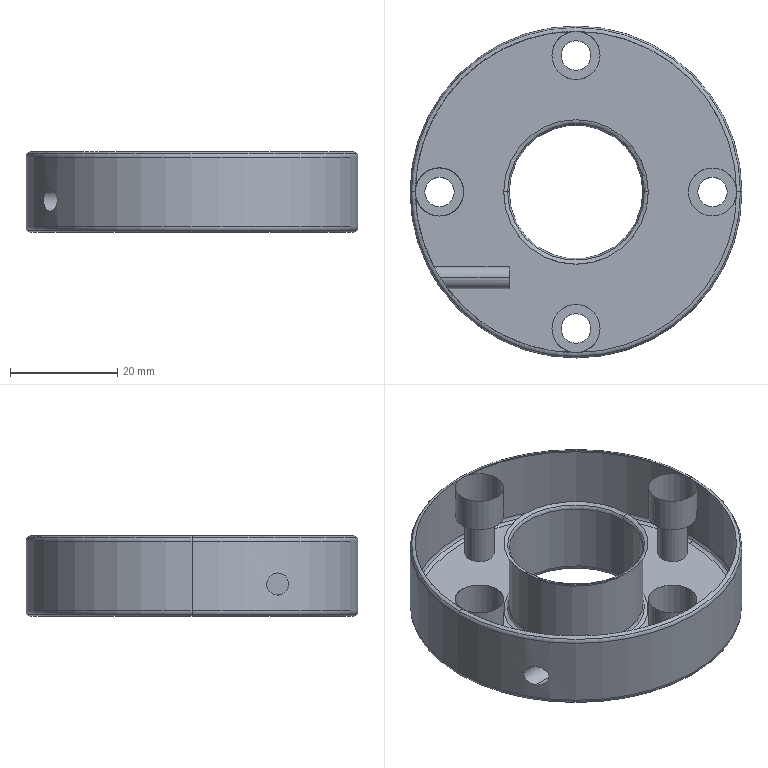Part | NX | features BREP 1 | 1 solid | 45 faces | box 62 x 62 x 15 mm | volume 35156 mm3 | cylinder 22 | torus 16 | plane 7 | commonest cylinder face diameters 5.5 x8 9 x8 4.134 x2 25 x2 62 x2
STEP:
#1=CARTESIAN_POINT('',(4.5,25.5,-6.5));
#2=VERTEX_POINT('',#1);
#3=CARTESIAN_POINT('',(-4.5,25.5,-6.5));
#4=VERTEX_POINT('',#3);
#5=CARTESIAN_POINT('',(0.,25.5,-6.5));
#6=DIRECTION('',(0.,0.,1.));
#7=DIRECTION('',(1.,0.,0.));
#8=AXIS2_PLACEMENT_3D('',#5,#6,#7);
#9=CIRCLE('',#8,4.5);
#10=EDGE_CURVE('',#2,#4,#9,.T.);
#11=ORIENTED_EDGE('',*,*,#10,.T.);
#12=CARTESIAN_POINT('',(0.,25.5,-6.5));
#13=DIRECTION('',(0.,0.,1.));
#14=DIRECTION('',(-1.,0.,0.));
#15=AXIS2_PLACEMENT_3D('',#12,#13,#14);
#16=CIRCLE('',#15,4.5);
#17=EDGE_CURVE('',#4,#2,#16,.T.);
#18=ORIENTED_EDGE('',*,*,#17,.T.);
#19=EDGE_LOOP('',(#11,#18));
#20=FACE_BOUND('',#19,.T.);
#21=CARTESIAN_POINT('',(2.75,25.5,-6.5));
#22=VERTEX_POINT('',#21);
#23=CARTESIAN_POINT('',(-2.75,25.5,-6.5));
#24=VERTEX_POINT('',#23);
#25=CARTESIAN_POINT('',(0.,25.5,-6.5));
#26=DIRECTION('',(0.,0.,-1.));
#27=DIRECTION('',(1.,0.,0.));
#28=AXIS2_PLACEMENT_3D('',#25,#26,#27);
#29=CIRCLE('',#28,2.75);
#30=EDGE_CURVE('',#22,#24,#29,.T.);
#31=ORIENTED_EDGE('',*,*,#30,.T.);
#32=CARTESIAN_POINT('',(0.,25.5,-6.5));
#33=DIRECTION('',(0.,0.,-1.));
#34=DIRECTION('',(-1.,0.,0.));
#35=AXIS2_PLACEMENT_3D('',#32,#33,#34);
#36=CIRCLE('',#35,2.75);
#37=EDGE_CURVE('',#24,#22,#36,.T.);
#38=ORIENTED_EDGE('',*,*,#37,.T.);
#39=EDGE_LOOP('',(#31,#38));
#40=FACE_BOUND('',#39,.T.);
#41=CARTESIAN_POINT('',(0.,30.,-6.5));
#42=DIRECTION('',(0.,0.,1.));
#43=DIRECTION('',(1.,0.,0.));
#44=AXIS2_PLACEMENT_3D('',#41,#42,#43);
#45=PLANE('',#44);
#46=ADVANCED_FACE('',(#20,#40),#45,.T.);
#47=CARTESIAN_POINT('',(4.5,25.5,0.));
#48=VERTEX_POINT('',#47);
#49=CARTESIAN_POINT('',(4.5,25.5,-6.5));
#50=DIRECTION('',(-0.000000009,-0.000000315,1.));
#51=VECTOR('',#50,1000.);
#52=LINE('',#49,#51);
#53=EDGE_CURVE('',#48,#2,#52,.F.);
#54=ORIENTED_EDGE('',*,*,#53,.T.);
#55=ORIENTED_EDGE('',*,*,#17,.F.);
#56=CARTESIAN_POINT('',(-4.5,25.5,0.));
#57=VERTEX_POINT('',#56);
#58=CARTESIAN_POINT('',(-4.5,25.5,-6.5));
#59=DIRECTION('',(0.,0.,1.));
#60=VECTOR('',#59,1000.);
#61=LINE('',#58,#60);
#62=EDGE_CURVE('',#57,#4,#61,.F.);
#63=ORIENTED_EDGE('',*,*,#62,.F.);
#64=CARTESIAN_POINT('',(0.,25.5,0.));
#65=DIRECTION('',(0.,0.,-1.));
#66=DIRECTION('',(1.,-0.000001366,0.));
#67=AXIS2_PLACEMENT_3D('',#64,#65,#66);
#68=CIRCLE('',#67,4.5);
#69=EDGE_CURVE('',#48,#57,#68,.T.);
#70=ORIENTED_EDGE('',*,*,#69,.F.);
#71=EDGE_LOOP('',(#54,#55,#63,#70));
#72=FACE_BOUND('',#71,.T.);
#73=CARTESIAN_POINT('',(0.,25.5,-6.5));
#74=DIRECTION('',(0.,0.,1.));
#75=DIRECTION('',(-1.,0.,0.));
#76=AXIS2_PLACEMENT_3D('',#73,#74,#75);
#77=CYLINDRICAL_SURFACE('',#76,4.5);
#78=ADVANCED_FACE('',(#72),#77,.F.);
#79=CARTESIAN_POINT('',(0.,30.,0.));
#80=VERTEX_POINT('',#79);
#81=CARTESIAN_POINT('',(0.,25.5,0.));
#82=DIRECTION('',(0.,0.,-1.));
#83=DIRECTION('',(-1.,0.,0.));
#84=AXIS2_PLACEMENT_3D('',#81,#82,#83);
#85=CIRCLE('',#84,4.5);
#86=EDGE_CURVE('',#57,#80,#85,.T.);
#87=ORIENTED_EDGE('',*,*,#86,.T.);
#88=CARTESIAN_POINT('',(-30.,0.,0.));
#89=VERTEX_POINT('',#88);
#90=CARTESIAN_POINT('',(0.,0.,0.));
#91=DIRECTION('',(0.,0.,1.));
#92=DIRECTION('',(0.,1.,0.));
#93=AXIS2_PLACEMENT_3D('',#90,#91,#92);
#94=CIRCLE('',#93,30.);
#95=EDGE_CURVE('',#80,#89,#94,.T.);
#96=ORIENTED_EDGE('',*,*,#95,.T.);
#97=CARTESIAN_POINT('',(-21.,0.,0.));
#98=VERTEX_POINT('',#97);
#99=CARTESIAN_POINT('',(-25.5,0.,0.));
#100=DIRECTION('',(0.,0.,-1.));
#101=DIRECTION('',(-1.,0.,0.));
#102=AXIS2_PLACEMENT_3D('',#99,#100,#101);
#103=CIRCLE('',#102,4.5);
#104=EDGE_CURVE('',#89,#98,#103,.T.);
#105=ORIENTED_EDGE('',*,*,#104,.T.);
#106=CARTESIAN_POINT('',(-25.5,0.,0.));
#107=DIRECTION('',(0.,0.,-1.));
#108=DIRECTION('',(1.,0.,0.));
#109=AXIS2_PLACEMENT_3D('',#106,#107,#108);
#110=CIRCLE('',#109,4.5);
#111=EDGE_CURVE('',#98,#89,#110,.T.);
#112=ORIENTED_EDGE('',*,*,#111,.T.);
#113=CARTESIAN_POINT('',(0.,-30.,0.));
#114=VERTEX_POINT('',#113);
#115=CARTESIAN_POINT('',(0.,0.,0.));
#116=DIRECTION('',(0.,0.,1.));
#117=DIRECTION('',(-1.,0.,0.));
#118=AXIS2_PLACEMENT_3D('',#115,#116,#117);
#119=CIRCLE('',#118,30.);
#120=EDGE_CURVE('',#89,#114,#119,.T.);
#121=ORIENTED_EDGE('',*,*,#120,.T.);
#122=CARTESIAN_POINT('',(-4.5,-25.5,0.));
#123=VERTEX_POINT('',#122);
#124=CARTESIAN_POINT('',(0.,-25.5,0.));
#125=DIRECTION('',(0.,0.,-1.));
#126=DIRECTION('',(0.,-1.,0.));
#127=AXIS2_PLACEMENT_3D('',#124,#125,#126);
#128=CIRCLE('',#127,4.5);
#129=EDGE_CURVE('',#114,#123,#128,.T.);
#130=ORIENTED_EDGE('',*,*,#129,.T.);
#131=CARTESIAN_POINT('',(4.5,-25.5,0.));
#132=VERTEX_POINT('',#131);
#133=CARTESIAN_POINT('',(0.,-25.5,0.));
#134=DIRECTION('',(0.,0.,-1.));
#135=DIRECTION('',(-1.,0.,0.));
#136=AXIS2_PLACEMENT_3D('',#133,#134,#135);
#137=CIRCLE('',#136,4.5);
#138=EDGE_CURVE('',#123,#132,#137,.T.);
#139=ORIENTED_EDGE('',*,*,#138,.T.);
#140=CARTESIAN_POINT('',(0.,-25.5,0.));
#141=DIRECTION('',(0.,0.,-1.));
#142=DIRECTION('',(1.,0.,0.));
#143=AXIS2_PLACEMENT_3D('',#140,#141,#142);
#144=CIRCLE('',#143,4.5);
#145=EDGE_CURVE('',#132,#114,#144,.T.);
#146=ORIENTED_EDGE('',*,*,#145,.T.);
#147=CARTESIAN_POINT('',(30.,0.,0.));
#148=VERTEX_POINT('',#147);
#149=CARTESIAN_POINT('',(0.,0.,0.));
#150=DIRECTION('',(0.,0.,1.));
#151=DIRECTION('',(0.,-1.,0.));
#152=AXIS2_PLACEMENT_3D('',#149,#150,#151);
#153=CIRCLE('',#152,30.);
#154=EDGE_CURVE('',#114,#148,#153,.T.);
#155=ORIENTED_EDGE('',*,*,#154,.T.);
#156=CARTESIAN_POINT('',(21.,0.,0.));
#157=VERTEX_POINT('',#156);
#158=CARTESIAN_POINT('',(25.5,0.,0.));
#159=DIRECTION('',(0.,0.,-1.));
#160=DIRECTION('',(1.,0.,0.));
#161=AXIS2_PLACEMENT_3D('',#158,#159,#160);
#162=CIRCLE('',#161,4.5);
#163=EDGE_CURVE('',#148,#157,#162,.T.);
#164=ORIENTED_EDGE('',*,*,#163,.T.);
#165=CARTESIAN_POINT('',(25.5,0.,0.));
#166=DIRECTION('',(0.,0.,-1.));
#167=DIRECTION('',(-1.,0.,0.));
#168=AXIS2_PLACEMENT_3D('',#165,#166,#167);
#169=CIRCLE('',#168,4.5);
#170=EDGE_CURVE('',#157,#148,#169,.T.);
#171=ORIENTED_EDGE('',*,*,#170,.T.);
#172=CARTESIAN_POINT('',(0.,0.,0.));
#173=DIRECTION('',(0.,0.,1.));
#174=DIRECTION('',(1.,0.,0.));
#175=AXIS2_PLACEMENT_3D('',#172,#173,#174);
#176=CIRCLE('',#175,30.);
#177=EDGE_CURVE('',#148,#80,#176,.T.);
#178=ORIENTED_EDGE('',*,*,#177,.T.);
#179=CARTESIAN_POINT('',(0.,25.5,0.));
#180=DIRECTION('',(0.,0.,-1.));
#181=DIRECTION('',(0.,1.,0.));
#182=AXIS2_PLACEMENT_3D('',#179,#180,#181);
#183=CIRCLE('',#182,4.5);
#184=EDGE_CURVE('',#80,#48,#183,.T.);
#185=ORIENTED_EDGE('',*,*,#184,.T.);
#186=ORIENTED_EDGE('',*,*,#69,.T.);
#187=EDGE_LOOP('',(#87,#96,#105,#112,#121,#130,#139,#146,#155,#164,#171,#178,#185,#186));
#188=FACE_BOUND('',#187,.T.);
#189=CARTESIAN_POINT('',(13.5,0.,0.));
#190=VERTEX_POINT('',#189);
#191=CARTESIAN_POINT('',(-13.5,0.,0.));
#192=VERTEX_POINT('',#191);
#193=CARTESIAN_POINT('',(0.,0.,0.));
#194=DIRECTION('',(0.,0.,-1.));
#195=DIRECTION('',(1.,0.,0.));
#196=AXIS2_PLACEMENT_3D('',#193,#194,#195);
#197=CIRCLE('',#196,13.5);
#198=EDGE_CURVE('',#190,#192,#197,.T.);
#199=ORIENTED_EDGE('',*,*,#198,.T.);
#200=CARTESIAN_POINT('',(0.,0.,0.));
#201=DIRECTION('',(0.,0.,-1.));
#202=DIRECTION('',(-1.,0.,0.));
#203=AXIS2_PLACEMENT_3D('',#200,#201,#202);
#204=CIRCLE('',#203,13.5);
#205=EDGE_CURVE('',#192,#190,#204,.T.);
#206=ORIENTED_EDGE('',*,*,#205,.T.);
#207=EDGE_LOOP('',(#199,#206));
#208=FACE_BOUND('',#207,.T.);
#209=CARTESIAN_POINT('',(0.,30.,0.));
#210=DIRECTION('',(0.,0.,1.));
#211=DIRECTION('',(1.,0.,0.));
#212=AXIS2_PLACEMENT_3D('',#209,#210,#211);
#213=PLANE('',#212);
#214=ADVANCED_FACE('',(#188,#208),#213,.T.);
#215=ORIENTED_EDGE('',*,*,#62,.T.);
#216=ORIENTED_EDGE('',*,*,#10,.F.);
#217=ORIENTED_EDGE('',*,*,#53,.F.);
#218=ORIENTED_EDGE('',*,*,#184,.F.);
#219=ORIENTED_EDGE('',*,*,#86,.F.);
#220=EDGE_LOOP('',(#215,#216,#217,#218,#219));
#221=FACE_BOUND('',#220,.T.);
#222=CARTESIAN_POINT('',(0.,25.5,-6.5));
#223=DIRECTION('',(0.,0.,1.));
#224=DIRECTION('',(-1.,0.,0.));
#225=AXIS2_PLACEMENT_3D('',#222,#223,#224);
#226=CYLINDRICAL_SURFACE('',#225,4.5);
#227=ADVANCED_FACE('',(#221),#226,.F.);
#228=ORIENTED_EDGE('',*,*,#177,.F.);
#229=CARTESIAN_POINT('',(30.707,0.,-0.2929));
#230=VERTEX_POINT('',#229);
#231=CARTESIAN_POINT('',(30.,0.,-1.));
#232=DIRECTION('',(0.,1.,0.));
#233=DIRECTION('',(0.,0.,1.));
#234=AXIS2_PLACEMENT_3D('',#231,#232,#233);
#235=CIRCLE('',#234,1.);
#236=EDGE_CURVE('',#230,#148,#235,.F.);
#237=ORIENTED_EDGE('',*,*,#236,.F.);
#238=CARTESIAN_POINT('',(-30.707,0.,-0.2929));
#239=VERTEX_POINT('',#238);
#240=CARTESIAN_POINT('',(0.,0.,-0.2929));
#241=DIRECTION('',(0.,0.,-1.));
#242=DIRECTION('',(-1.,0.,0.));
#243=AXIS2_PLACEMENT_3D('',#240,#241,#242);
#244=CIRCLE('',#243,30.707);
#245=EDGE_CURVE('',#239,#230,#244,.T.);
#246=ORIENTED_EDGE('',*,*,#245,.F.);
#247=CARTESIAN_POINT('',(-30.,0.,-1.));
#248=DIRECTION('',(0.,-1.,0.));
#249=DIRECTION('',(0.,0.,1.));
#250=AXIS2_PLACEMENT_3D('',#247,#248,#249);
#251=CIRCLE('',#250,1.);
#252=EDGE_CURVE('',#239,#89,#251,.F.);
#253=ORIENTED_EDGE('',*,*,#252,.T.);
#254=ORIENTED_EDGE('',*,*,#95,.F.);
#255=EDGE_LOOP('',(#228,#237,#246,#253,#254));
#256=FACE_BOUND('',#255,.T.);
#257=CARTESIAN_POINT('',(0.,0.,-1.));
#258=DIRECTION('',(0.,0.,-1.));
#259=DIRECTION('',(-1.,0.,0.));
#260=AXIS2_PLACEMENT_3D('',#257,#258,#259);
#261=TOROIDAL_SURFACE('',#260,30.,1.);
#262=ADVANCED_FACE('',(#256),#261,.T.);
#263=ORIENTED_EDGE('',*,*,#120,.F.);
#264=ORIENTED_EDGE('',*,*,#252,.F.);
#265=CARTESIAN_POINT('',(0.,0.,-0.2929));
#266=DIRECTION('',(0.,0.,-1.));
#267=DIRECTION('',(1.,0.,0.));
#268=AXIS2_PLACEMENT_3D('',#265,#266,#267);
#269=CIRCLE('',#268,30.707);
#270=EDGE_CURVE('',#230,#239,#269,.T.);
#271=ORIENTED_EDGE('',*,*,#270,.F.);
#272=ORIENTED_EDGE('',*,*,#236,.T.);
#273=ORIENTED_EDGE('',*,*,#154,.F.);
#274=EDGE_LOOP('',(#263,#264,#271,#272,#273));
#275=FACE_BOUND('',#274,.T.);
#276=CARTESIAN_POINT('',(0.,0.,-1.));
#277=DIRECTION('',(0.,0.,-1.));
#278=DIRECTION('',(-1.,0.,0.));
#279=AXIS2_PLACEMENT_3D('',#276,#277,#278);
#280=TOROIDAL_SURFACE('',#279,30.,1.);
#281=ADVANCED_FACE('',(#275),#280,.T.);
#282=CARTESIAN_POINT('',(31.,0.,-1.));
#283=VERTEX_POINT('',#282);
#284=CARTESIAN_POINT('',(30.,0.,-1.));
#285=DIRECTION('',(0.,1.,0.));
#286=DIRECTION('',(0.7071,0.,0.7071));
#287=AXIS2_PLACEMENT_3D('',#284,#285,#286);
#288=CIRCLE('',#287,1.);
#289=EDGE_CURVE('',#283,#230,#288,.F.);
#290=ORIENTED_EDGE('',*,*,#289,.T.);
#291=ORIENTED_EDGE('',*,*,#270,.T.);
#292=CARTESIAN_POINT('',(-31.,0.,-1.));
#293=VERTEX_POINT('',#292);
#294=CARTESIAN_POINT('',(-30.,0.,-1.));
#295=DIRECTION('',(0.,-1.,0.));
#296=DIRECTION('',(-0.7071,0.,0.7071));
#297=AXIS2_PLACEMENT_3D('',#294,#295,#296);
#298=CIRCLE('',#297,1.);
#299=EDGE_CURVE('',#293,#239,#298,.F.);
#300=ORIENTED_EDGE('',*,*,#299,.F.);
#301=CARTESIAN_POINT('',(0.,0.,-1.));
#302=DIRECTION('',(0.,0.,1.));
#303=DIRECTION('',(-1.,0.,0.));
#304=AXIS2_PLACEMENT_3D('',#301,#302,#303);
#305=CIRCLE('',#304,31.);
#306=EDGE_CURVE('',#293,#283,#305,.T.);
#307=ORIENTED_EDGE('',*,*,#306,.T.);
#308=EDGE_LOOP('',(#290,#291,#300,#307));
#309=FACE_BOUND('',#308,.T.);
#310=CARTESIAN_POINT('',(0.,0.,-1.));
#311=DIRECTION('',(0.,0.,-1.));
#312=DIRECTION('',(-1.,0.,0.));
#313=AXIS2_PLACEMENT_3D('',#310,#311,#312);
#314=TOROIDAL_SURFACE('',#313,30.,1.);
#315=ADVANCED_FACE('',(#309),#314,.T.);
#316=CARTESIAN_POINT('',(31.,0.,-14.));
#317=VERTEX_POINT('',#316);
#318=CARTESIAN_POINT('',(31.,0.,-14.));
#319=DIRECTION('',(0.,0.,1.));
#320=VECTOR('',#319,1000.);
#321=LINE('',#318,#320);
#322=EDGE_CURVE('',#283,#317,#321,.F.);
#323=ORIENTED_EDGE('',*,*,#322,.F.);
#324=ORIENTED_EDGE('',*,*,#306,.F.);
#325=CARTESIAN_POINT('',(-31.,0.,-14.));
#326=VERTEX_POINT('',#325);
#327=CARTESIAN_POINT('',(-31.,0.,-14.));
#328=DIRECTION('',(0.,0.,1.));
#329=VECTOR('',#328,1000.);
#330=LINE('',#327,#329);
#331=EDGE_CURVE('',#293,#326,#330,.F.);
#332=ORIENTED_EDGE('',*,*,#331,.T.);
#333=CARTESIAN_POINT('',(0.,0.,-14.));
#334=DIRECTION('',(0.,0.,-1.));
#335=DIRECTION('',(1.,0.,0.));
#336=AXIS2_PLACEMENT_3D('',#333,#334,#335);
#337=CIRCLE('',#336,31.);
#338=EDGE_CURVE('',#317,#326,#337,.T.);
#339=ORIENTED_EDGE('',*,*,#338,.F.);
#340=EDGE_LOOP('',(#323,#324,#332,#339));
#341=FACE_BOUND('',#340,.T.);
#342=CARTESIAN_POINT('',(-26.552,-16.,-11.067));
#343=VERTEX_POINT('',#342);
#344=CARTESIAN_POINT('',(-26.506,-16.075,-11.066));
#345=VERTEX_POINT('',#344);
#346=CARTESIAN_POINT('',(-26.552,-16.,-11.067));
#347=CARTESIAN_POINT('',(-26.547,-16.008,-11.067));
#348=CARTESIAN_POINT('',(-26.537,-16.025,-11.067));
#349=CARTESIAN_POINT('',(-26.521,-16.05,-11.066));
#350=CARTESIAN_POINT('',(-26.511,-16.067,-11.066));
#351=CARTESIAN_POINT('',(-26.506,-16.075,-11.066));
#352=B_SPLINE_CURVE_WITH_KNOTS('',3,(#346,#347,#348,#349,#350,#351),.UNSPECIFIED.,.F.,.F.,(4,1,1,4),(0.,0.3333,0.6667,1.),.UNSPECIFIED.);
#353=EDGE_CURVE('',#343,#345,#352,.T.);
#354=ORIENTED_EDGE('',*,*,#353,.F.);
#355=CARTESIAN_POINT('',(-26.552,-16.,-6.933));
#356=VERTEX_POINT('',#355);
#357=CARTESIAN_POINT('',(-26.552,-16.,-11.067));
#358=CARTESIAN_POINT('',(-26.906,-15.413,-11.067));
#359=CARTESIAN_POINT('',(-27.511,-14.308,-10.535));
#360=CARTESIAN_POINT('',(-27.784,-13.744,-8.997));
#361=CARTESIAN_POINT('',(-27.507,-14.315,-7.458));
#362=CARTESIAN_POINT('',(-26.903,-15.417,-6.933));
#363=CARTESIAN_POINT('',(-26.552,-16.,-6.933));
#364=B_SPLINE_CURVE_WITH_KNOTS('',3,(#357,#358,#359,#360,#361,#362,#363),.UNSPECIFIED.,.F.,.F.,(4,1,1,1,4),(0.,0.25,0.5,0.75,1.),.UNSPECIFIED.);
#365=EDGE_CURVE('',#356,#343,#364,.F.);
#366=ORIENTED_EDGE('',*,*,#365,.F.);
#367=CARTESIAN_POINT('',(-26.552,-16.,-6.933));
#368=CARTESIAN_POINT('',(-26.198,-16.588,-6.933));
#369=CARTESIAN_POINT('',(-25.449,-17.721,-7.498));
#370=CARTESIAN_POINT('',(-25.069,-18.23,-8.97));
#371=CARTESIAN_POINT('',(-25.421,-17.758,-10.451));
#372=CARTESIAN_POINT('',(-26.15,-16.662,-11.044));
#373=CARTESIAN_POINT('',(-26.506,-16.075,-11.066));
#374=B_SPLINE_CURVE_WITH_KNOTS('',3,(#367,#368,#369,#370,#371,#372,#373),.UNSPECIFIED.,.F.,.F.,(4,1,1,1,4),(0.,0.25,0.5,0.75,1.),.UNSPECIFIED.);
#375=EDGE_CURVE('',#345,#356,#374,.F.);
#376=ORIENTED_EDGE('',*,*,#375,.F.);
#377=EDGE_LOOP('',(#354,#366,#376));
#378=FACE_BOUND('',#377,.T.);
#379=CARTESIAN_POINT('',(0.,0.,-50.));
#380=DIRECTION('',(0.,0.,1.));
#381=DIRECTION('',(-1.,0.,0.));
#382=AXIS2_PLACEMENT_3D('',#379,#380,#381);
#383=CYLINDRICAL_SURFACE('',#382,31.);
#384=ADVANCED_FACE('',(#341,#378),#383,.T.);
#385=CARTESIAN_POINT('',(-30.707,0.,-14.707));
#386=VERTEX_POINT('',#385);
#387=CARTESIAN_POINT('',(-30.,0.,-14.));
#388=DIRECTION('',(0.,-1.,0.));
#389=DIRECTION('',(-1.,0.,0.));
#390=AXIS2_PLACEMENT_3D('',#387,#388,#389);
#391=CIRCLE('',#390,1.);
#392=EDGE_CURVE('',#326,#386,#391,.T.);
#393=ORIENTED_EDGE('',*,*,#392,.T.);
#394=CARTESIAN_POINT('',(30.707,0.,-14.707));
#395=VERTEX_POINT('',#394);
#396=CARTESIAN_POINT('',(0.,0.,-14.707));
#397=DIRECTION('',(0.,0.,-1.));
#398=DIRECTION('',(1.,0.,0.));
#399=AXIS2_PLACEMENT_3D('',#396,#397,#398);
#400=CIRCLE('',#399,30.707);
#401=EDGE_CURVE('',#395,#386,#400,.T.);
#402=ORIENTED_EDGE('',*,*,#401,.F.);
#403=CARTESIAN_POINT('',(30.,0.,-14.));
#404=DIRECTION('',(0.,1.,0.));
#405=DIRECTION('',(1.,0.,0.));
#406=AXIS2_PLACEMENT_3D('',#403,#404,#405);
#407=CIRCLE('',#406,1.);
#408=EDGE_CURVE('',#317,#395,#407,.T.);
#409=ORIENTED_EDGE('',*,*,#408,.F.);
#410=ORIENTED_EDGE('',*,*,#338,.T.);
#411=EDGE_LOOP('',(#393,#402,#409,#410));
#412=FACE_BOUND('',#411,.T.);
#413=CARTESIAN_POINT('',(0.,0.,-14.));
#414=DIRECTION('',(0.,0.,-1.));
#415=DIRECTION('',(-1.,0.,0.));
#416=AXIS2_PLACEMENT_3D('',#413,#414,#415);
#417=TOROIDAL_SURFACE('',#416,30.,1.);
#418=ADVANCED_FACE('',(#412),#417,.T.);
#419=ORIENTED_EDGE('',*,*,#408,.T.);
#420=CARTESIAN_POINT('',(0.,0.,-14.707));
#421=DIRECTION('',(0.,0.,-1.));
#422=DIRECTION('',(-1.,0.,0.));
#423=AXIS2_PLACEMENT_3D('',#420,#421,#422);
#424=CIRCLE('',#423,30.707);
#425=EDGE_CURVE('',#386,#395,#424,.T.);
#426=ORIENTED_EDGE('',*,*,#425,.F.);
#427=ORIENTED_EDGE('',*,*,#392,.F.);
#428=CARTESIAN_POINT('',(0.,0.,-14.));
#429=DIRECTION('',(0.,0.,-1.));
#430=DIRECTION('',(-1.,0.,0.));
#431=AXIS2_PLACEMENT_3D('',#428,#429,#430);
#432=CIRCLE('',#431,31.);
#433=EDGE_CURVE('',#326,#317,#432,.T.);
#434=ORIENTED_EDGE('',*,*,#433,.T.);
#435=EDGE_LOOP('',(#419,#426,#427,#434));
#436=FACE_BOUND('',#435,.T.);
#437=CARTESIAN_POINT('',(0.,0.,-14.));
#438=DIRECTION('',(0.,0.,-1.));
#439=DIRECTION('',(-1.,0.,0.));
#440=AXIS2_PLACEMENT_3D('',#437,#438,#439);
#441=TOROIDAL_SURFACE('',#440,30.,1.);
#442=ADVANCED_FACE('',(#436),#441,.T.);
#443=ORIENTED_EDGE('',*,*,#331,.F.);
#444=CARTESIAN_POINT('',(0.,0.,-1.));
#445=DIRECTION('',(0.,0.,1.));
#446=DIRECTION('',(1.,0.,0.));
#447=AXIS2_PLACEMENT_3D('',#444,#445,#446);
#448=CIRCLE('',#447,31.);
#449=EDGE_CURVE('',#283,#293,#448,.T.);
#450=ORIENTED_EDGE('',*,*,#449,.F.);
#451=ORIENTED_EDGE('',*,*,#322,.T.);
#452=ORIENTED_EDGE('',*,*,#433,.F.);
#453=EDGE_LOOP('',(#443,#450,#451,#452));
#454=FACE_BOUND('',#453,.T.);
#455=CARTESIAN_POINT('',(0.,0.,-50.));
#456=DIRECTION('',(0.,0.,1.));
#457=DIRECTION('',(-1.,0.,0.));
#458=AXIS2_PLACEMENT_3D('',#455,#456,#457);
#459=CYLINDRICAL_SURFACE('',#458,31.);
#460=ADVANCED_FACE('',(#454),#459,.T.);
#461=ORIENTED_EDGE('',*,*,#299,.T.);
#462=ORIENTED_EDGE('',*,*,#245,.T.);
#463=ORIENTED_EDGE('',*,*,#289,.F.);
#464=ORIENTED_EDGE('',*,*,#449,.T.);
#465=EDGE_LOOP('',(#461,#462,#463,#464));
#466=FACE_BOUND('',#465,.T.);
#467=CARTESIAN_POINT('',(0.,0.,-1.));
#468=DIRECTION('',(0.,0.,-1.));
#469=DIRECTION('',(-1.,0.,0.));
#470=AXIS2_PLACEMENT_3D('',#467,#468,#469);
#471=TOROIDAL_SURFACE('',#470,30.,1.);
#472=ADVANCED_FACE('',(#466),#471,.T.);
#473=CARTESIAN_POINT('',(-30.,0.,-15.));
#474=VERTEX_POINT('',#473);
#475=CARTESIAN_POINT('',(-30.,0.,-14.));
#476=DIRECTION('',(0.,-1.,0.));
#477=DIRECTION('',(-0.7071,0.,-0.7071));
#478=AXIS2_PLACEMENT_3D('',#475,#476,#477);
#479=CIRCLE('',#478,1.);
#480=EDGE_CURVE('',#386,#474,#479,.T.);
#481=ORIENTED_EDGE('',*,*,#480,.F.);
#482=ORIENTED_EDGE('',*,*,#425,.T.);
#483=CARTESIAN_POINT('',(30.,0.,-15.));
#484=VERTEX_POINT('',#483);
#485=CARTESIAN_POINT('',(30.,0.,-14.));
#486=DIRECTION('',(0.,1.,0.));
#487=DIRECTION('',(0.7071,0.,-0.7071));
#488=AXIS2_PLACEMENT_3D('',#485,#486,#487);
#489=CIRCLE('',#488,1.);
#490=EDGE_CURVE('',#395,#484,#489,.T.);
#491=ORIENTED_EDGE('',*,*,#490,.T.);
#492=CARTESIAN_POINT('',(0.,0.,-15.));
#493=DIRECTION('',(0.,0.,-1.));
#494=DIRECTION('',(-1.,0.,0.));
#495=AXIS2_PLACEMENT_3D('',#492,#493,#494);
#496=CIRCLE('',#495,30.);
#497=EDGE_CURVE('',#474,#484,#496,.T.);
#498=ORIENTED_EDGE('',*,*,#497,.F.);
#499=EDGE_LOOP('',(#481,#482,#491,#498));
#500=FACE_BOUND('',#499,.T.);
#501=CARTESIAN_POINT('',(0.,0.,-14.));
#502=DIRECTION('',(0.,0.,-1.));
#503=DIRECTION('',(-1.,0.,0.));
#504=AXIS2_PLACEMENT_3D('',#501,#502,#503);
#505=TOROIDAL_SURFACE('',#504,30.,1.);
#506=ADVANCED_FACE('',(#500),#505,.T.);
#507=CARTESIAN_POINT('',(0.,0.,-15.));
#508=DIRECTION('',(0.,0.,-1.));
#509=DIRECTION('',(1.,0.,0.));
#510=AXIS2_PLACEMENT_3D('',#507,#508,#509);
#511=CIRCLE('',#510,30.);
#512=EDGE_CURVE('',#484,#474,#511,.T.);
#513=ORIENTED_EDGE('',*,*,#512,.T.);
#514=ORIENTED_EDGE('',*,*,#497,.T.);
#515=EDGE_LOOP('',(#513,#514));
#516=FACE_BOUND('',#515,.T.);
#517=CARTESIAN_POINT('',(2.75,25.5,-15.));
#518=VERTEX_POINT('',#517);
#519=CARTESIAN_POINT('',(-2.75,25.5,-15.));
#520=VERTEX_POINT('',#519);
#521=CARTESIAN_POINT('',(0.,25.5,-15.));
#522=DIRECTION('',(0.,0.,1.));
#523=DIRECTION('',(1.,0.,0.));
#524=AXIS2_PLACEMENT_3D('',#521,#522,#523);
#525=CIRCLE('',#524,2.75);
#526=EDGE_CURVE('',#518,#520,#525,.T.);
#527=ORIENTED_EDGE('',*,*,#526,.T.);
#528=CARTESIAN_POINT('',(0.,25.5,-15.));
#529=DIRECTION('',(0.,0.,1.));
#530=DIRECTION('',(-1.,0.,0.));
#531=AXIS2_PLACEMENT_3D('',#528,#529,#530);
#532=CIRCLE('',#531,2.75);
#533=EDGE_CURVE('',#520,#518,#532,.T.);
#534=ORIENTED_EDGE('',*,*,#533,.T.);
#535=EDGE_LOOP('',(#527,#534));
#536=FACE_BOUND('',#535,.T.);
#537=CARTESIAN_POINT('',(-22.75,0.,-15.));
#538=VERTEX_POINT('',#537);
#539=CARTESIAN_POINT('',(-28.25,0.,-15.));
#540=VERTEX_POINT('',#539);
#541=CARTESIAN_POINT('',(-25.5,0.,-15.));
#542=DIRECTION('',(0.,0.,1.));
#543=DIRECTION('',(1.,0.,0.));
#544=AXIS2_PLACEMENT_3D('',#541,#542,#543);
#545=CIRCLE('',#544,2.75);
#546=EDGE_CURVE('',#538,#540,#545,.T.);
#547=ORIENTED_EDGE('',*,*,#546,.T.);
#548=CARTESIAN_POINT('',(-25.5,0.,-15.));
#549=DIRECTION('',(0.,0.,1.));
#550=DIRECTION('',(-1.,0.,0.));
#551=AXIS2_PLACEMENT_3D('',#548,#549,#550);
#552=CIRCLE('',#551,2.75);
#553=EDGE_CURVE('',#540,#538,#552,.T.);
#554=ORIENTED_EDGE('',*,*,#553,.T.);
#555=EDGE_LOOP('',(#547,#554));
#556=FACE_BOUND('',#555,.T.);
#557=CARTESIAN_POINT('',(28.25,0.,-15.));
#558=VERTEX_POINT('',#557);
#559=CARTESIAN_POINT('',(22.75,0.,-15.));
#560=VERTEX_POINT('',#559);
#561=CARTESIAN_POINT('',(25.5,0.,-15.));
#562=DIRECTION('',(0.,0.,1.));
#563=DIRECTION('',(1.,0.,0.));
#564=AXIS2_PLACEMENT_3D('',#561,#562,#563);
#565=CIRCLE('',#564,2.75);
#566=EDGE_CURVE('',#558,#560,#565,.T.);
#567=ORIENTED_EDGE('',*,*,#566,.T.);
#568=CARTESIAN_POINT('',(25.5,0.,-15.));
#569=DIRECTION('',(0.,0.,1.));
#570=DIRECTION('',(-1.,0.,0.));
#571=AXIS2_PLACEMENT_3D('',#568,#569,#570);
#572=CIRCLE('',#571,2.75);
#573=EDGE_CURVE('',#560,#558,#572,.T.);
#574=ORIENTED_EDGE('',*,*,#573,.T.);
#575=EDGE_LOOP('',(#567,#574));
#576=FACE_BOUND('',#575,.T.);
#577=CARTESIAN_POINT('',(-2.75,-25.5,-15.));
#578=VERTEX_POINT('',#577);
#579=CARTESIAN_POINT('',(2.75,-25.5,-15.));
#580=VERTEX_POINT('',#579);
#581=CARTESIAN_POINT('',(0.,-25.5,-15.));
#582=DIRECTION('',(0.,0.,1.));
#583=DIRECTION('',(-1.,0.,0.));
#584=AXIS2_PLACEMENT_3D('',#581,#582,#583);
#585=CIRCLE('',#584,2.75);
#586=EDGE_CURVE('',#578,#580,#585,.T.);
#587=ORIENTED_EDGE('',*,*,#586,.T.);
#588=CARTESIAN_POINT('',(0.,-25.5,-15.));
#589=DIRECTION('',(0.,0.,1.));
#590=DIRECTION('',(1.,0.,0.));
#591=AXIS2_PLACEMENT_3D('',#588,#589,#590);
#592=CIRCLE('',#591,2.75);
#593=EDGE_CURVE('',#580,#578,#592,.T.);
#594=ORIENTED_EDGE('',*,*,#593,.T.);
#595=EDGE_LOOP('',(#587,#594));
#596=FACE_BOUND('',#595,.T.);
#597=CARTESIAN_POINT('',(13.5,0.,-15.));
#598=VERTEX_POINT('',#597);
#599=CARTESIAN_POINT('',(-13.5,0.,-15.));
#600=VERTEX_POINT('',#599);
#601=CARTESIAN_POINT('',(0.,0.,-15.));
#602=DIRECTION('',(0.,0.,1.));
#603=DIRECTION('',(1.,0.,0.));
#604=AXIS2_PLACEMENT_3D('',#601,#602,#603);
#605=CIRCLE('',#604,13.5);
#606=EDGE_CURVE('',#598,#600,#605,.T.);
#607=ORIENTED_EDGE('',*,*,#606,.T.);
#608=CARTESIAN_POINT('',(0.,0.,-15.));
#609=DIRECTION('',(0.,0.,1.));
#610=DIRECTION('',(-1.,0.,0.));
#611=AXIS2_PLACEMENT_3D('',#608,#609,#610);
#612=CIRCLE('',#611,13.5);
#613=EDGE_CURVE('',#600,#598,#612,.T.);
#614=ORIENTED_EDGE('',*,*,#613,.T.);
#615=EDGE_LOOP('',(#607,#614));
#616=FACE_BOUND('',#615,.T.);
#617=CARTESIAN_POINT('',(0.,13.5,-15.));
#618=DIRECTION('',(0.,0.,-1.));
#619=DIRECTION('',(0.,-1.,0.));
#620=AXIS2_PLACEMENT_3D('',#617,#618,#619);
#621=PLANE('',#620);
#622=ADVANCED_FACE('',(#516,#536,#556,#576,#596,#616),#621,.T.);
#623=ORIENTED_EDGE('',*,*,#490,.F.);
#624=ORIENTED_EDGE('',*,*,#401,.T.);
#625=ORIENTED_EDGE('',*,*,#480,.T.);
#626=ORIENTED_EDGE('',*,*,#512,.F.);
#627=EDGE_LOOP('',(#623,#624,#625,#626));
#628=FACE_BOUND('',#627,.T.);
#629=CARTESIAN_POINT('',(0.,0.,-14.));
#630=DIRECTION('',(0.,0.,-1.));
#631=DIRECTION('',(-1.,0.,0.));
#632=AXIS2_PLACEMENT_3D('',#629,#630,#631);
#633=TOROIDAL_SURFACE('',#632,30.,1.);
#634=ADVANCED_FACE('',(#628),#633,.T.);
#635=CARTESIAN_POINT('',(2.75,25.5,-15.));
#636=DIRECTION('',(0.,0.,1.));
#637=VECTOR('',#636,1000.);
#638=LINE('',#635,#637);
#639=EDGE_CURVE('',#22,#518,#638,.F.);
#640=ORIENTED_EDGE('',*,*,#639,.T.);
#641=ORIENTED_EDGE('',*,*,#533,.F.);
#642=CARTESIAN_POINT('',(-2.75,25.5,-15.));
#643=DIRECTION('',(0.,0.,1.));
#644=VECTOR('',#643,1000.);
#645=LINE('',#642,#644);
#646=EDGE_CURVE('',#24,#520,#645,.F.);
#647=ORIENTED_EDGE('',*,*,#646,.F.);
#648=ORIENTED_EDGE('',*,*,#30,.F.);
#649=EDGE_LOOP('',(#640,#641,#647,#648));
#650=FACE_BOUND('',#649,.T.);
#651=CARTESIAN_POINT('',(0.,25.5,-6.5));
#652=DIRECTION('',(0.,0.,1.));
#653=DIRECTION('',(-1.,0.,0.));
#654=AXIS2_PLACEMENT_3D('',#651,#652,#653);
#655=CYLINDRICAL_SURFACE('',#654,2.75);
#656=ADVANCED_FACE('',(#650),#655,.F.);
#657=ORIENTED_EDGE('',*,*,#646,.T.);
#658=ORIENTED_EDGE('',*,*,#526,.F.);
#659=ORIENTED_EDGE('',*,*,#639,.F.);
#660=ORIENTED_EDGE('',*,*,#37,.F.);
#661=EDGE_LOOP('',(#657,#658,#659,#660));
#662=FACE_BOUND('',#661,.T.);
#663=CARTESIAN_POINT('',(0.,25.5,-6.5));
#664=DIRECTION('',(0.,0.,1.));
#665=DIRECTION('',(-1.,0.,0.));
#666=AXIS2_PLACEMENT_3D('',#663,#664,#665);
#667=CYLINDRICAL_SURFACE('',#666,2.75);
#668=ADVANCED_FACE('',(#662),#667,.F.);
#669=CARTESIAN_POINT('',(-22.75,0.,-6.5));
#670=VERTEX_POINT('',#669);
#671=CARTESIAN_POINT('',(-22.75,0.,-15.));
#672=DIRECTION('',(0.,0.,1.));
#673=VECTOR('',#672,1000.);
#674=LINE('',#671,#673);
#675=EDGE_CURVE('',#670,#538,#674,.F.);
#676=ORIENTED_EDGE('',*,*,#675,.T.);
#677=ORIENTED_EDGE('',*,*,#553,.F.);
#678=CARTESIAN_POINT('',(-28.25,0.,-6.5));
#679=VERTEX_POINT('',#678);
#680=CARTESIAN_POINT('',(-28.25,0.,-15.));
#681=DIRECTION('',(0.,0.,1.));
#682=VECTOR('',#681,1000.);
#683=LINE('',#680,#682);
#684=EDGE_CURVE('',#679,#540,#683,.F.);
#685=ORIENTED_EDGE('',*,*,#684,.F.);
#686=CARTESIAN_POINT('',(-25.5,0.,-6.5));
#687=DIRECTION('',(0.,0.,-1.));
#688=DIRECTION('',(1.,0.,0.));
#689=AXIS2_PLACEMENT_3D('',#686,#687,#688);
#690=CIRCLE('',#689,2.75);
#691=EDGE_CURVE('',#670,#679,#690,.T.);
#692=ORIENTED_EDGE('',*,*,#691,.F.);
#693=EDGE_LOOP('',(#676,#677,#685,#692));
#694=FACE_BOUND('',#693,.T.);
#695=CARTESIAN_POINT('',(-25.5,0.,-6.5));
#696=DIRECTION('',(0.,0.,1.));
#697=DIRECTION('',(-1.,0.,0.));
#698=AXIS2_PLACEMENT_3D('',#695,#696,#697);
#699=CYLINDRICAL_SURFACE('',#698,2.75);
#700=ADVANCED_FACE('',(#694),#699,.F.);
#701=CARTESIAN_POINT('',(-21.,0.,-6.5));
#702=VERTEX_POINT('',#701);
#703=CARTESIAN_POINT('',(-30.,0.,-6.5));
#704=VERTEX_POINT('',#703);
#705=CARTESIAN_POINT('',(-25.5,0.,-6.5));
#706=DIRECTION('',(0.,0.,1.));
#707=DIRECTION('',(1.,0.,0.));
#708=AXIS2_PLACEMENT_3D('',#705,#706,#707);
#709=CIRCLE('',#708,4.5);
#710=EDGE_CURVE('',#702,#704,#709,.T.);
#711=ORIENTED_EDGE('',*,*,#710,.T.);
#712=CARTESIAN_POINT('',(-25.5,0.,-6.5));
#713=DIRECTION('',(0.,0.,1.));
#714=DIRECTION('',(-1.,0.,0.));
#715=AXIS2_PLACEMENT_3D('',#712,#713,#714);
#716=CIRCLE('',#715,4.5);
#717=EDGE_CURVE('',#704,#702,#716,.T.);
#718=ORIENTED_EDGE('',*,*,#717,.T.);
#719=EDGE_LOOP('',(#711,#718));
#720=FACE_BOUND('',#719,.T.);
#721=ORIENTED_EDGE('',*,*,#691,.T.);
#722=CARTESIAN_POINT('',(-25.5,0.,-6.5));
#723=DIRECTION('',(0.,0.,-1.));
#724=DIRECTION('',(-1.,0.,0.));
#725=AXIS2_PLACEMENT_3D('',#722,#723,#724);
#726=CIRCLE('',#725,2.75);
#727=EDGE_CURVE('',#679,#670,#726,.T.);
#728=ORIENTED_EDGE('',*,*,#727,.T.);
#729=EDGE_LOOP('',(#721,#728));
#730=FACE_BOUND('',#729,.T.);
#731=CARTESIAN_POINT('',(-30.,0.,-6.5));
#732=DIRECTION('',(0.,0.,1.));
#733=DIRECTION('',(1.,0.,0.));
#734=AXIS2_PLACEMENT_3D('',#731,#732,#733);
#735=PLANE('',#734);
#736=ADVANCED_FACE('',(#720,#730),#735,.T.);
#737=CARTESIAN_POINT('',(-21.,0.,-6.5));
#738=DIRECTION('',(0.,0.,1.));
#739=VECTOR('',#738,1000.);
#740=LINE('',#737,#739);
#741=EDGE_CURVE('',#98,#702,#740,.F.);
#742=ORIENTED_EDGE('',*,*,#741,.T.);
#743=ORIENTED_EDGE('',*,*,#717,.F.);
#744=CARTESIAN_POINT('',(-30.,0.,-6.5));
#745=DIRECTION('',(0.,0.,1.));
#746=VECTOR('',#745,1000.);
#747=LINE('',#744,#746);
#748=EDGE_CURVE('',#89,#704,#747,.F.);
#749=ORIENTED_EDGE('',*,*,#748,.F.);
#750=ORIENTED_EDGE('',*,*,#111,.F.);
#751=EDGE_LOOP('',(#742,#743,#749,#750));
#752=FACE_BOUND('',#751,.T.);
#753=CARTESIAN_POINT('',(-25.5,0.,-6.5));
#754=DIRECTION('',(0.,0.,1.));
#755=DIRECTION('',(-1.,0.,0.));
#756=AXIS2_PLACEMENT_3D('',#753,#754,#755);
#757=CYLINDRICAL_SURFACE('',#756,4.5);
#758=ADVANCED_FACE('',(#752),#757,.F.);
#759=ORIENTED_EDGE('',*,*,#748,.T.);
#760=ORIENTED_EDGE('',*,*,#710,.F.);
#761=ORIENTED_EDGE('',*,*,#741,.F.);
#762=ORIENTED_EDGE('',*,*,#104,.F.);
#763=EDGE_LOOP('',(#759,#760,#761,#762));
#764=FACE_BOUND('',#763,.T.);
#765=CARTESIAN_POINT('',(-25.5,0.,-6.5));
#766=DIRECTION('',(0.,0.,1.));
#767=DIRECTION('',(-1.,0.,0.));
#768=AXIS2_PLACEMENT_3D('',#765,#766,#767);
#769=CYLINDRICAL_SURFACE('',#768,4.5);
#770=ADVANCED_FACE('',(#764),#769,.F.);
#771=ORIENTED_EDGE('',*,*,#684,.T.);
#772=ORIENTED_EDGE('',*,*,#546,.F.);
#773=ORIENTED_EDGE('',*,*,#675,.F.);
#774=ORIENTED_EDGE('',*,*,#727,.F.);
#775=EDGE_LOOP('',(#771,#772,#773,#774));
#776=FACE_BOUND('',#775,.T.);
#777=CARTESIAN_POINT('',(-25.5,0.,-6.5));
#778=DIRECTION('',(0.,0.,1.));
#779=DIRECTION('',(-1.,0.,0.));
#780=AXIS2_PLACEMENT_3D('',#777,#778,#779);
#781=CYLINDRICAL_SURFACE('',#780,2.75);
#782=ADVANCED_FACE('',(#776),#781,.F.);
#783=CARTESIAN_POINT('',(28.25,0.,-6.5));
#784=VERTEX_POINT('',#783);
#785=CARTESIAN_POINT('',(28.25,0.,-15.));
#786=DIRECTION('',(0.,0.,1.));
#787=VECTOR('',#786,1000.);
#788=LINE('',#785,#787);
#789=EDGE_CURVE('',#784,#558,#788,.F.);
#790=ORIENTED_EDGE('',*,*,#789,.T.);
#791=ORIENTED_EDGE('',*,*,#573,.F.);
#792=CARTESIAN_POINT('',(22.75,0.,-6.5));
#793=VERTEX_POINT('',#792);
#794=CARTESIAN_POINT('',(22.75,0.,-15.));
#795=DIRECTION('',(0.,0.,1.));
#796=VECTOR('',#795,1000.);
#797=LINE('',#794,#796);
#798=EDGE_CURVE('',#793,#560,#797,.F.);
#799=ORIENTED_EDGE('',*,*,#798,.F.);
#800=CARTESIAN_POINT('',(25.5,0.,-6.5));
#801=DIRECTION('',(0.,0.,-1.));
#802=DIRECTION('',(1.,0.,0.));
#803=AXIS2_PLACEMENT_3D('',#800,#801,#802);
#804=CIRCLE('',#803,2.75);
#805=EDGE_CURVE('',#784,#793,#804,.T.);
#806=ORIENTED_EDGE('',*,*,#805,.F.);
#807=EDGE_LOOP('',(#790,#791,#799,#806));
#808=FACE_BOUND('',#807,.T.);
#809=CARTESIAN_POINT('',(25.5,0.,-6.5));
#810=DIRECTION('',(0.,0.,1.));
#811=DIRECTION('',(-1.,0.,0.));
#812=AXIS2_PLACEMENT_3D('',#809,#810,#811);
#813=CYLINDRICAL_SURFACE('',#812,2.75);
#814=ADVANCED_FACE('',(#808),#813,.F.);
#815=CARTESIAN_POINT('',(30.,0.,-6.5));
#816=VERTEX_POINT('',#815);
#817=CARTESIAN_POINT('',(21.,0.,-6.5));
#818=VERTEX_POINT('',#817);
#819=CARTESIAN_POINT('',(25.5,0.,-6.5));
#820=DIRECTION('',(0.,0.,1.));
#821=DIRECTION('',(1.,0.,0.));
#822=AXIS2_PLACEMENT_3D('',#819,#820,#821);
#823=CIRCLE('',#822,4.5);
#824=EDGE_CURVE('',#816,#818,#823,.T.);
#825=ORIENTED_EDGE('',*,*,#824,.T.);
#826=CARTESIAN_POINT('',(25.5,0.,-6.5));
#827=DIRECTION('',(0.,0.,1.));
#828=DIRECTION('',(-1.,0.,0.));
#829=AXIS2_PLACEMENT_3D('',#826,#827,#828);
#830=CIRCLE('',#829,4.5);
#831=EDGE_CURVE('',#818,#816,#830,.T.);
#832=ORIENTED_EDGE('',*,*,#831,.T.);
#833=EDGE_LOOP('',(#825,#832));
#834=FACE_BOUND('',#833,.T.);
#835=ORIENTED_EDGE('',*,*,#805,.T.);
#836=CARTESIAN_POINT('',(25.5,0.,-6.5));
#837=DIRECTION('',(0.,0.,-1.));
#838=DIRECTION('',(-1.,0.,0.));
#839=AXIS2_PLACEMENT_3D('',#836,#837,#838);
#840=CIRCLE('',#839,2.75);
#841=EDGE_CURVE('',#793,#784,#840,.T.);
#842=ORIENTED_EDGE('',*,*,#841,.T.);
#843=EDGE_LOOP('',(#835,#842));
#844=FACE_BOUND('',#843,.T.);
#845=CARTESIAN_POINT('',(21.,0.,-6.5));
#846=DIRECTION('',(0.,0.,1.));
#847=DIRECTION('',(1.,0.,0.));
#848=AXIS2_PLACEMENT_3D('',#845,#846,#847);
#849=PLANE('',#848);
#850=ADVANCED_FACE('',(#834,#844),#849,.T.);
#851=CARTESIAN_POINT('',(30.,0.,-6.5));
#852=DIRECTION('',(0.,0.,1.));
#853=VECTOR('',#852,1000.);
#854=LINE('',#851,#853);
#855=EDGE_CURVE('',#148,#816,#854,.F.);
#856=ORIENTED_EDGE('',*,*,#855,.T.);
#857=ORIENTED_EDGE('',*,*,#831,.F.);
#858=CARTESIAN_POINT('',(21.,0.,-6.5));
#859=DIRECTION('',(0.,0.,1.));
#860=VECTOR('',#859,1000.);
#861=LINE('',#858,#860);
#862=EDGE_CURVE('',#157,#818,#861,.F.);
#863=ORIENTED_EDGE('',*,*,#862,.F.);
#864=ORIENTED_EDGE('',*,*,#163,.F.);
#865=EDGE_LOOP('',(#856,#857,#863,#864));
#866=FACE_BOUND('',#865,.T.);
#867=CARTESIAN_POINT('',(25.5,0.,-6.5));
#868=DIRECTION('',(0.,0.,1.));
#869=DIRECTION('',(-1.,0.,0.));
#870=AXIS2_PLACEMENT_3D('',#867,#868,#869);
#871=CYLINDRICAL_SURFACE('',#870,4.5);
#872=ADVANCED_FACE('',(#866),#871,.F.);
#873=ORIENTED_EDGE('',*,*,#862,.T.);
#874=ORIENTED_EDGE('',*,*,#824,.F.);
#875=ORIENTED_EDGE('',*,*,#855,.F.);
#876=ORIENTED_EDGE('',*,*,#170,.F.);
#877=EDGE_LOOP('',(#873,#874,#875,#876));
#878=FACE_BOUND('',#877,.T.);
#879=CARTESIAN_POINT('',(25.5,0.,-6.5));
#880=DIRECTION('',(0.,0.,1.));
#881=DIRECTION('',(-1.,0.,0.));
#882=AXIS2_PLACEMENT_3D('',#879,#880,#881);
#883=CYLINDRICAL_SURFACE('',#882,4.5);
#884=ADVANCED_FACE('',(#878),#883,.F.);
#885=ORIENTED_EDGE('',*,*,#798,.T.);
#886=ORIENTED_EDGE('',*,*,#566,.F.);
#887=ORIENTED_EDGE('',*,*,#789,.F.);
#888=ORIENTED_EDGE('',*,*,#841,.F.);
#889=EDGE_LOOP('',(#885,#886,#887,#888));
#890=FACE_BOUND('',#889,.T.);
#891=CARTESIAN_POINT('',(25.5,0.,-6.5));
#892=DIRECTION('',(0.,0.,1.));
#893=DIRECTION('',(-1.,0.,0.));
#894=AXIS2_PLACEMENT_3D('',#891,#892,#893);
#895=CYLINDRICAL_SURFACE('',#894,2.75);
#896=ADVANCED_FACE('',(#890),#895,.F.);
#897=CARTESIAN_POINT('',(2.75,-25.5,-6.5));
#898=VERTEX_POINT('',#897);
#899=CARTESIAN_POINT('',(2.75,-25.5,-6.5));
#900=DIRECTION('',(0.,0.,-1.));
#901=VECTOR('',#900,1000.);
#902=LINE('',#899,#901);
#903=EDGE_CURVE('',#580,#898,#902,.F.);
#904=ORIENTED_EDGE('',*,*,#903,.T.);
#905=CARTESIAN_POINT('',(-2.75,-25.5,-6.5));
#906=VERTEX_POINT('',#905);
#907=CARTESIAN_POINT('',(0.,-25.5,-6.5));
#908=DIRECTION('',(0.,0.,-1.));
#909=DIRECTION('',(-1.,0.,0.));
#910=AXIS2_PLACEMENT_3D('',#907,#908,#909);
#911=CIRCLE('',#910,2.75);
#912=EDGE_CURVE('',#906,#898,#911,.T.);
#913=ORIENTED_EDGE('',*,*,#912,.F.);
#914=CARTESIAN_POINT('',(-2.75,-25.5,-6.5));
#915=DIRECTION('',(0.,0.,-1.));
#916=VECTOR('',#915,1000.);
#917=LINE('',#914,#916);
#918=EDGE_CURVE('',#578,#906,#917,.F.);
#919=ORIENTED_EDGE('',*,*,#918,.F.);
#920=ORIENTED_EDGE('',*,*,#593,.F.);
#921=EDGE_LOOP('',(#904,#913,#919,#920));
#922=FACE_BOUND('',#921,.T.);
#923=CARTESIAN_POINT('',(0.,-25.5,0.));
#924=DIRECTION('',(0.,0.,-1.));
#925=DIRECTION('',(1.,0.,0.));
#926=AXIS2_PLACEMENT_3D('',#923,#924,#925);
#927=CYLINDRICAL_SURFACE('',#926,2.75);
#928=ADVANCED_FACE('',(#922),#927,.F.);
#929=ORIENTED_EDGE('',*,*,#918,.T.);
#930=CARTESIAN_POINT('',(0.,-25.5,-6.5));
#931=DIRECTION('',(0.,0.,-1.));
#932=DIRECTION('',(1.,0.,0.));
#933=AXIS2_PLACEMENT_3D('',#930,#931,#932);
#934=CIRCLE('',#933,2.75);
#935=EDGE_CURVE('',#898,#906,#934,.T.);
#936=ORIENTED_EDGE('',*,*,#935,.F.);
#937=ORIENTED_EDGE('',*,*,#903,.F.);
#938=ORIENTED_EDGE('',*,*,#586,.F.);
#939=EDGE_LOOP('',(#929,#936,#937,#938));
#940=FACE_BOUND('',#939,.T.);
#941=CARTESIAN_POINT('',(0.,-25.5,0.));
#942=DIRECTION('',(0.,0.,-1.));
#943=DIRECTION('',(1.,0.,0.));
#944=AXIS2_PLACEMENT_3D('',#941,#942,#943);
#945=CYLINDRICAL_SURFACE('',#944,2.75);
#946=ADVANCED_FACE('',(#940),#945,.F.);
#947=CARTESIAN_POINT('',(-4.5,-25.5,-6.5));
#948=VERTEX_POINT('',#947);
#949=CARTESIAN_POINT('',(4.5,-25.5,-6.5));
#950=VERTEX_POINT('',#949);
#951=CARTESIAN_POINT('',(0.,-25.5,-6.5));
#952=DIRECTION('',(0.,0.,1.));
#953=DIRECTION('',(-1.,0.,0.));
#954=AXIS2_PLACEMENT_3D('',#951,#952,#953);
#955=CIRCLE('',#954,4.5);
#956=EDGE_CURVE('',#948,#950,#955,.T.);
#957=ORIENTED_EDGE('',*,*,#956,.T.);
#958=CARTESIAN_POINT('',(0.,-25.5,-6.5));
#959=DIRECTION('',(0.,0.,1.));
#960=DIRECTION('',(1.,0.,0.));
#961=AXIS2_PLACEMENT_3D('',#958,#959,#960);
#962=CIRCLE('',#961,4.5);
#963=EDGE_CURVE('',#950,#948,#962,.T.);
#964=ORIENTED_EDGE('',*,*,#963,.T.);
#965=EDGE_LOOP('',(#957,#964));
#966=FACE_BOUND('',#965,.T.);
#967=ORIENTED_EDGE('',*,*,#912,.T.);
#968=ORIENTED_EDGE('',*,*,#935,.T.);
#969=EDGE_LOOP('',(#967,#968));
#970=FACE_BOUND('',#969,.T.);
#971=CARTESIAN_POINT('',(0.,-28.25,-6.5));
#972=DIRECTION('',(0.,0.,1.));
#973=DIRECTION('',(1.,0.,0.));
#974=AXIS2_PLACEMENT_3D('',#971,#972,#973);
#975=PLANE('',#974);
#976=ADVANCED_FACE('',(#966,#970),#975,.T.);
#977=CARTESIAN_POINT('',(4.5,-25.5,0.));
#978=DIRECTION('',(0.00000005,0.,-1.));
#979=VECTOR('',#978,1000.);
#980=LINE('',#977,#979);
#981=EDGE_CURVE('',#950,#132,#980,.F.);
#982=ORIENTED_EDGE('',*,*,#981,.T.);
#983=ORIENTED_EDGE('',*,*,#138,.F.);
#984=CARTESIAN_POINT('',(-4.5,-25.5,0.));
#985=DIRECTION('',(0.,0.,-1.));
#986=VECTOR('',#985,1000.);
#987=LINE('',#984,#986);
#988=EDGE_CURVE('',#948,#123,#987,.F.);
#989=ORIENTED_EDGE('',*,*,#988,.F.);
#990=ORIENTED_EDGE('',*,*,#963,.F.);
#991=EDGE_LOOP('',(#982,#983,#989,#990));
#992=FACE_BOUND('',#991,.T.);
#993=CARTESIAN_POINT('',(0.,-25.5,0.));
#994=DIRECTION('',(0.,0.,-1.));
#995=DIRECTION('',(1.,0.,0.));
#996=AXIS2_PLACEMENT_3D('',#993,#994,#995);
#997=CYLINDRICAL_SURFACE('',#996,4.5);
#998=ADVANCED_FACE('',(#992),#997,.F.);
#999=ORIENTED_EDGE('',*,*,#988,.T.);
#1000=ORIENTED_EDGE('',*,*,#129,.F.);
#1001=ORIENTED_EDGE('',*,*,#145,.F.);
#1002=ORIENTED_EDGE('',*,*,#981,.F.);
#1003=ORIENTED_EDGE('',*,*,#956,.F.);
#1004=EDGE_LOOP('',(#999,#1000,#1001,#1002,#1003));
#1005=FACE_BOUND('',#1004,.T.);
#1006=CARTESIAN_POINT('',(0.,-25.5,0.));
#1007=DIRECTION('',(0.,0.,-1.));
#1008=DIRECTION('',(1.,0.,0.));
#1009=AXIS2_PLACEMENT_3D('',#1006,#1007,#1008);
#1010=CYLINDRICAL_SURFACE('',#1009,4.5);
#1011=ADVANCED_FACE('',(#1005),#1010,.F.);
#1012=CARTESIAN_POINT('',(-12.793,0.,-14.707));
#1013=VERTEX_POINT('',#1012);
#1014=CARTESIAN_POINT('',(-13.5,0.,-14.));
#1015=DIRECTION('',(0.,-1.,0.));
#1016=DIRECTION('',(0.,0.,-1.));
#1017=AXIS2_PLACEMENT_3D('',#1014,#1015,#1016);
#1018=CIRCLE('',#1017,1.);
#1019=EDGE_CURVE('',#600,#1013,#1018,.T.);
#1020=ORIENTED_EDGE('',*,*,#1019,.T.);
#1021=CARTESIAN_POINT('',(12.793,0.,-14.707));
#1022=VERTEX_POINT('',#1021);
#1023=CARTESIAN_POINT('',(0.,0.,-14.707));
#1024=DIRECTION('',(0.,0.,-1.));
#1025=DIRECTION('',(1.,0.,0.));
#1026=AXIS2_PLACEMENT_3D('',#1023,#1024,#1025);
#1027=CIRCLE('',#1026,12.793);
#1028=EDGE_CURVE('',#1022,#1013,#1027,.T.);
#1029=ORIENTED_EDGE('',*,*,#1028,.F.);
#1030=CARTESIAN_POINT('',(13.5,0.,-14.));
#1031=DIRECTION('',(0.,1.,0.));
#1032=DIRECTION('',(0.,0.,-1.));
#1033=AXIS2_PLACEMENT_3D('',#1030,#1031,#1032);
#1034=CIRCLE('',#1033,1.);
#1035=EDGE_CURVE('',#598,#1022,#1034,.T.);
#1036=ORIENTED_EDGE('',*,*,#1035,.F.);
#1037=ORIENTED_EDGE('',*,*,#613,.F.);
#1038=EDGE_LOOP('',(#1020,#1029,#1036,#1037));
#1039=FACE_BOUND('',#1038,.T.);
#1040=CARTESIAN_POINT('',(0.,0.,-14.));
#1041=DIRECTION('',(0.,0.,-1.));
#1042=DIRECTION('',(-1.,0.,0.));
#1043=AXIS2_PLACEMENT_3D('',#1040,#1041,#1042);
#1044=TOROIDAL_SURFACE('',#1043,13.5,1.);
#1045=ADVANCED_FACE('',(#1039),#1044,.T.);
#1046=ORIENTED_EDGE('',*,*,#1035,.T.);
#1047=CARTESIAN_POINT('',(0.,0.,-14.707));
#1048=DIRECTION('',(0.,0.,-1.));
#1049=DIRECTION('',(-1.,0.,0.));
#1050=AXIS2_PLACEMENT_3D('',#1047,#1048,#1049);
#1051=CIRCLE('',#1050,12.793);
#1052=EDGE_CURVE('',#1013,#1022,#1051,.T.);
#1053=ORIENTED_EDGE('',*,*,#1052,.F.);
#1054=ORIENTED_EDGE('',*,*,#1019,.F.);
#1055=ORIENTED_EDGE('',*,*,#606,.F.);
#1056=EDGE_LOOP('',(#1046,#1053,#1054,#1055));
#1057=FACE_BOUND('',#1056,.T.);
#1058=CARTESIAN_POINT('',(0.,0.,-14.));
#1059=DIRECTION('',(0.,0.,-1.));
#1060=DIRECTION('',(-1.,0.,0.));
#1061=AXIS2_PLACEMENT_3D('',#1058,#1059,#1060);
#1062=TOROIDAL_SURFACE('',#1061,13.5,1.);
#1063=ADVANCED_FACE('',(#1057),#1062,.T.);
#1064=CARTESIAN_POINT('',(-12.5,0.,-14.));
#1065=VERTEX_POINT('',#1064);
#1066=CARTESIAN_POINT('',(-13.5,0.,-14.));
#1067=DIRECTION('',(0.,-1.,0.));
#1068=DIRECTION('',(0.7071,0.,-0.7071));
#1069=AXIS2_PLACEMENT_3D('',#1066,#1067,#1068);
#1070=CIRCLE('',#1069,1.);
#1071=EDGE_CURVE('',#1013,#1065,#1070,.T.);
#1072=ORIENTED_EDGE('',*,*,#1071,.F.);
#1073=ORIENTED_EDGE('',*,*,#1052,.T.);
#1074=CARTESIAN_POINT('',(12.5,0.,-14.));
#1075=VERTEX_POINT('',#1074);
#1076=CARTESIAN_POINT('',(13.5,0.,-14.));
#1077=DIRECTION('',(0.,1.,0.));
#1078=DIRECTION('',(-0.7071,0.,-0.7071));
#1079=AXIS2_PLACEMENT_3D('',#1076,#1077,#1078);
#1080=CIRCLE('',#1079,1.);
#1081=EDGE_CURVE('',#1022,#1075,#1080,.T.);
#1082=ORIENTED_EDGE('',*,*,#1081,.T.);
#1083=CARTESIAN_POINT('',(0.,0.,-14.));
#1084=DIRECTION('',(0.,0.,1.));
#1085=DIRECTION('',(1.,0.,0.));
#1086=AXIS2_PLACEMENT_3D('',#1083,#1084,#1085);
#1087=CIRCLE('',#1086,12.5);
#1088=EDGE_CURVE('',#1075,#1065,#1087,.T.);
#1089=ORIENTED_EDGE('',*,*,#1088,.T.);
#1090=EDGE_LOOP('',(#1072,#1073,#1082,#1089));
#1091=FACE_BOUND('',#1090,.T.);
#1092=CARTESIAN_POINT('',(0.,0.,-14.));
#1093=DIRECTION('',(0.,0.,-1.));
#1094=DIRECTION('',(-1.,0.,0.));
#1095=AXIS2_PLACEMENT_3D('',#1092,#1093,#1094);
#1096=TOROIDAL_SURFACE('',#1095,13.5,1.);
#1097=ADVANCED_FACE('',(#1091),#1096,.T.);
#1098=CARTESIAN_POINT('',(-12.5,0.,-1.));
#1099=VERTEX_POINT('',#1098);
#1100=CARTESIAN_POINT('',(-12.5,0.,-14.));
#1101=DIRECTION('',(0.,0.,1.));
#1102=VECTOR('',#1101,1000.);
#1103=LINE('',#1100,#1102);
#1104=EDGE_CURVE('',#1065,#1099,#1103,.T.);
#1105=ORIENTED_EDGE('',*,*,#1104,.F.);
#1106=ORIENTED_EDGE('',*,*,#1088,.F.);
#1107=CARTESIAN_POINT('',(12.5,0.,-1.));
#1108=VERTEX_POINT('',#1107);
#1109=CARTESIAN_POINT('',(12.5,0.,-14.));
#1110=DIRECTION('',(0.,0.,1.));
#1111=VECTOR('',#1110,1000.);
#1112=LINE('',#1109,#1111);
#1113=EDGE_CURVE('',#1075,#1108,#1112,.T.);
#1114=ORIENTED_EDGE('',*,*,#1113,.T.);
#1115=CARTESIAN_POINT('',(0.,0.,-1.));
#1116=DIRECTION('',(0.,0.,-1.));
#1117=DIRECTION('',(-1.,0.,0.));
#1118=AXIS2_PLACEMENT_3D('',#1115,#1116,#1117);
#1119=CIRCLE('',#1118,12.5);
#1120=EDGE_CURVE('',#1099,#1108,#1119,.T.);
#1121=ORIENTED_EDGE('',*,*,#1120,.F.);
#1122=EDGE_LOOP('',(#1105,#1106,#1114,#1121));
#1123=FACE_BOUND('',#1122,.T.);
#1124=CARTESIAN_POINT('',(0.,0.,-50.));
#1125=DIRECTION('',(0.,0.,1.));
#1126=DIRECTION('',(-1.,0.,0.));
#1127=AXIS2_PLACEMENT_3D('',#1124,#1125,#1126);
#1128=CYLINDRICAL_SURFACE('',#1127,12.5);
#1129=ADVANCED_FACE('',(#1123),#1128,.F.);
#1130=CARTESIAN_POINT('',(12.793,0.,-0.2929));
#1131=VERTEX_POINT('',#1130);
#1132=CARTESIAN_POINT('',(13.5,0.,-1.));
#1133=DIRECTION('',(0.,1.,0.));
#1134=DIRECTION('',(-1.,0.,0.));
#1135=AXIS2_PLACEMENT_3D('',#1132,#1133,#1134);
#1136=CIRCLE('',#1135,1.);
#1137=EDGE_CURVE('',#1131,#1108,#1136,.F.);
#1138=ORIENTED_EDGE('',*,*,#1137,.F.);
#1139=CARTESIAN_POINT('',(-12.793,0.,-0.2929));
#1140=VERTEX_POINT('',#1139);
#1141=CARTESIAN_POINT('',(0.,0.,-0.2929));
#1142=DIRECTION('',(0.,0.,-1.));
#1143=DIRECTION('',(-1.,0.,0.));
#1144=AXIS2_PLACEMENT_3D('',#1141,#1142,#1143);
#1145=CIRCLE('',#1144,12.793);
#1146=EDGE_CURVE('',#1140,#1131,#1145,.T.);
#1147=ORIENTED_EDGE('',*,*,#1146,.F.);
#1148=CARTESIAN_POINT('',(-13.5,0.,-1.));
#1149=DIRECTION('',(0.,-1.,0.));
#1150=DIRECTION('',(1.,0.,0.));
#1151=AXIS2_PLACEMENT_3D('',#1148,#1149,#1150);
#1152=CIRCLE('',#1151,1.);
#1153=EDGE_CURVE('',#1140,#1099,#1152,.F.);
#1154=ORIENTED_EDGE('',*,*,#1153,.T.);
#1155=ORIENTED_EDGE('',*,*,#1120,.T.);
#1156=EDGE_LOOP('',(#1138,#1147,#1154,#1155));
#1157=FACE_BOUND('',#1156,.T.);
#1158=CARTESIAN_POINT('',(0.,0.,-1.));
#1159=DIRECTION('',(0.,0.,-1.));
#1160=DIRECTION('',(-1.,0.,0.));
#1161=AXIS2_PLACEMENT_3D('',#1158,#1159,#1160);
#1162=TOROIDAL_SURFACE('',#1161,13.5,1.);
#1163=ADVANCED_FACE('',(#1157),#1162,.T.);
#1164=ORIENTED_EDGE('',*,*,#1153,.F.);
#1165=CARTESIAN_POINT('',(0.,0.,-0.2929));
#1166=DIRECTION('',(0.,0.,-1.));
#1167=DIRECTION('',(1.,0.,0.));
#1168=AXIS2_PLACEMENT_3D('',#1165,#1166,#1167);
#1169=CIRCLE('',#1168,12.793);
#1170=EDGE_CURVE('',#1131,#1140,#1169,.T.);
#1171=ORIENTED_EDGE('',*,*,#1170,.F.);
#1172=ORIENTED_EDGE('',*,*,#1137,.T.);
#1173=CARTESIAN_POINT('',(0.,0.,-1.));
#1174=DIRECTION('',(0.,0.,-1.));
#1175=DIRECTION('',(1.,0.,0.));
#1176=AXIS2_PLACEMENT_3D('',#1173,#1174,#1175);
#1177=CIRCLE('',#1176,12.5);
#1178=EDGE_CURVE('',#1108,#1099,#1177,.T.);
#1179=ORIENTED_EDGE('',*,*,#1178,.T.);
#1180=EDGE_LOOP('',(#1164,#1171,#1172,#1179));
#1181=FACE_BOUND('',#1180,.T.);
#1182=CARTESIAN_POINT('',(0.,0.,-1.));
#1183=DIRECTION('',(0.,0.,-1.));
#1184=DIRECTION('',(-1.,0.,0.));
#1185=AXIS2_PLACEMENT_3D('',#1182,#1183,#1184);
#1186=TOROIDAL_SURFACE('',#1185,13.5,1.);
#1187=ADVANCED_FACE('',(#1181),#1186,.T.);
#1188=ORIENTED_EDGE('',*,*,#1113,.F.);
#1189=CARTESIAN_POINT('',(0.,0.,-14.));
#1190=DIRECTION('',(0.,0.,1.));
#1191=DIRECTION('',(-1.,0.,0.));
#1192=AXIS2_PLACEMENT_3D('',#1189,#1190,#1191);
#1193=CIRCLE('',#1192,12.5);
#1194=EDGE_CURVE('',#1065,#1075,#1193,.T.);
#1195=ORIENTED_EDGE('',*,*,#1194,.F.);
#1196=ORIENTED_EDGE('',*,*,#1104,.T.);
#1197=ORIENTED_EDGE('',*,*,#1178,.F.);
#1198=EDGE_LOOP('',(#1188,#1195,#1196,#1197));
#1199=FACE_BOUND('',#1198,.T.);
#1200=CARTESIAN_POINT('',(0.,0.,-50.));
#1201=DIRECTION('',(0.,0.,1.));
#1202=DIRECTION('',(-1.,0.,0.));
#1203=AXIS2_PLACEMENT_3D('',#1200,#1201,#1202);
#1204=CYLINDRICAL_SURFACE('',#1203,12.5);
#1205=ADVANCED_FACE('',(#1199),#1204,.F.);
#1206=ORIENTED_EDGE('',*,*,#1081,.F.);
#1207=ORIENTED_EDGE('',*,*,#1028,.T.);
#1208=ORIENTED_EDGE('',*,*,#1071,.T.);
#1209=ORIENTED_EDGE('',*,*,#1194,.T.);
#1210=EDGE_LOOP('',(#1206,#1207,#1208,#1209));
#1211=FACE_BOUND('',#1210,.T.);
#1212=CARTESIAN_POINT('',(0.,0.,-14.));
#1213=DIRECTION('',(0.,0.,-1.));
#1214=DIRECTION('',(-1.,0.,0.));
#1215=AXIS2_PLACEMENT_3D('',#1212,#1213,#1214);
#1216=TOROIDAL_SURFACE('',#1215,13.5,1.);
#1217=ADVANCED_FACE('',(#1211),#1216,.T.);
#1218=CARTESIAN_POINT('',(13.5,0.,-1.));
#1219=DIRECTION('',(0.,1.,0.));
#1220=DIRECTION('',(-0.7071,0.,0.7071));
#1221=AXIS2_PLACEMENT_3D('',#1218,#1219,#1220);
#1222=CIRCLE('',#1221,1.);
#1223=EDGE_CURVE('',#190,#1131,#1222,.F.);
#1224=ORIENTED_EDGE('',*,*,#1223,.T.);
#1225=ORIENTED_EDGE('',*,*,#1170,.T.);
#1226=CARTESIAN_POINT('',(-13.5,0.,-1.));
#1227=DIRECTION('',(0.,-1.,0.));
#1228=DIRECTION('',(0.7071,0.,0.7071));
#1229=AXIS2_PLACEMENT_3D('',#1226,#1227,#1228);
#1230=CIRCLE('',#1229,1.);
#1231=EDGE_CURVE('',#192,#1140,#1230,.F.);
#1232=ORIENTED_EDGE('',*,*,#1231,.F.);
#1233=ORIENTED_EDGE('',*,*,#198,.F.);
#1234=EDGE_LOOP('',(#1224,#1225,#1232,#1233));
#1235=FACE_BOUND('',#1234,.T.);
#1236=CARTESIAN_POINT('',(0.,0.,-1.));
#1237=DIRECTION('',(0.,0.,-1.));
#1238=DIRECTION('',(-1.,0.,0.));
#1239=AXIS2_PLACEMENT_3D('',#1236,#1237,#1238);
#1240=TOROIDAL_SURFACE('',#1239,13.5,1.);
#1241=ADVANCED_FACE('',(#1235),#1240,.T.);
#1242=ORIENTED_EDGE('',*,*,#1231,.T.);
#1243=ORIENTED_EDGE('',*,*,#1146,.T.);
#1244=ORIENTED_EDGE('',*,*,#1223,.F.);
#1245=ORIENTED_EDGE('',*,*,#205,.F.);
#1246=EDGE_LOOP('',(#1242,#1243,#1244,#1245));
#1247=FACE_BOUND('',#1246,.T.);
#1248=CARTESIAN_POINT('',(0.,0.,-1.));
#1249=DIRECTION('',(0.,0.,-1.));
#1250=DIRECTION('',(-1.,0.,0.));
#1251=AXIS2_PLACEMENT_3D('',#1248,#1249,#1250);
#1252=TOROIDAL_SURFACE('',#1251,13.5,1.);
#1253=ADVANCED_FACE('',(#1247),#1252,.T.);
#1254=CARTESIAN_POINT('',(-12.5,-16.,-11.067));
#1255=VERTEX_POINT('',#1254);
#1256=CARTESIAN_POINT('',(-26.552,-16.,-11.067));
#1257=DIRECTION('',(1.,0.,0.000000175));
#1258=VECTOR('',#1257,1000.);
#1259=LINE('',#1256,#1258);
#1260=EDGE_CURVE('',#343,#1255,#1259,.T.);
#1261=ORIENTED_EDGE('',*,*,#1260,.F.);
#1262=ORIENTED_EDGE('',*,*,#353,.T.);
#1263=ORIENTED_EDGE('',*,*,#375,.T.);
#1264=CARTESIAN_POINT('',(-12.5,-16.,-6.933));
#1265=VERTEX_POINT('',#1264);
#1266=CARTESIAN_POINT('',(-26.552,-16.,-6.933));
#1267=DIRECTION('',(1.,0.,0.));
#1268=VECTOR('',#1267,1000.);
#1269=LINE('',#1266,#1268);
#1270=EDGE_CURVE('',#356,#1265,#1269,.T.);
#1271=ORIENTED_EDGE('',*,*,#1270,.T.);
#1272=CARTESIAN_POINT('',(-12.5,-16.,-9.));
#1273=DIRECTION('',(-1.,0.,0.));
#1274=DIRECTION('',(0.,0.,-1.));
#1275=AXIS2_PLACEMENT_3D('',#1272,#1273,#1274);
#1276=CIRCLE('',#1275,2.067);
#1277=EDGE_CURVE('',#1255,#1265,#1276,.T.);
#1278=ORIENTED_EDGE('',*,*,#1277,.F.);
#1279=EDGE_LOOP('',(#1261,#1262,#1263,#1271,#1278));
#1280=FACE_BOUND('',#1279,.T.);
#1281=CARTESIAN_POINT('',(-29.5,-16.,-9.));
#1282=DIRECTION('',(1.,0.,0.));
#1283=DIRECTION('',(0.,0.,1.));
#1284=AXIS2_PLACEMENT_3D('',#1281,#1282,#1283);
#1285=CYLINDRICAL_SURFACE('',#1284,2.067);
#1286=ADVANCED_FACE('',(#1280),#1285,.F.);
#1287=ORIENTED_EDGE('',*,*,#1277,.T.);
#1288=CARTESIAN_POINT('',(-12.5,-16.,-9.));
#1289=DIRECTION('',(-1.,0.,0.));
#1290=DIRECTION('',(0.,0.,1.));
#1291=AXIS2_PLACEMENT_3D('',#1288,#1289,#1290);
#1292=CIRCLE('',#1291,2.067);
#1293=EDGE_CURVE('',#1265,#1255,#1292,.T.);
#1294=ORIENTED_EDGE('',*,*,#1293,.T.);
#1295=EDGE_LOOP('',(#1287,#1294));
#1296=FACE_BOUND('',#1295,.T.);
#1297=CARTESIAN_POINT('',(-12.5,-16.,-9.));
#1298=DIRECTION('',(-1.,0.,0.));
#1299=DIRECTION('',(0.,0.,1.));
#1300=AXIS2_PLACEMENT_3D('',#1297,#1298,#1299);
#1301=PLANE('',#1300);
#1302=ADVANCED_FACE('',(#1296),#1301,.T.);
#1303=ORIENTED_EDGE('',*,*,#1270,.F.);
#1304=ORIENTED_EDGE('',*,*,#365,.T.);
#1305=ORIENTED_EDGE('',*,*,#1260,.T.);
#1306=ORIENTED_EDGE('',*,*,#1293,.F.);
#1307=EDGE_LOOP('',(#1303,#1304,#1305,#1306));
#1308=FACE_BOUND('',#1307,.T.);
#1309=CARTESIAN_POINT('',(-29.5,-16.,-9.));
#1310=DIRECTION('',(1.,0.,0.));
#1311=DIRECTION('',(0.,0.,1.));
#1312=AXIS2_PLACEMENT_3D('',#1309,#1310,#1311);
#1313=CYLINDRICAL_SURFACE('',#1312,2.067);
#1314=ADVANCED_FACE('',(#1308),#1313,.F.);
#1315=CLOSED_SHELL('',(#46,#78,#214,#227,#262,#281,#315,#384,#418,#442,#460,#472,#506,#622,#634,#656,#668,#700,#736,#758,#770,#782,#814,#850,#872,#884,#896,#928,#946,#976,#998,#1011,#1045,#1063,#1097,#1129,#1163,#1187,#1205,#1217,#1241,#1253,#1286,#1302,#1314));
#1316=MANIFOLD_SOLID_BREP('',#1315);
#1317=(LENGTH_UNIT()NAMED_UNIT(*)SI_UNIT(.MILLI.,.METRE.));
#1318=UNCERTAINTY_MEASURE_WITH_UNIT(LENGTH_MEASURE(0.0508),#1317,'','');
#1319=(NAMED_UNIT(*)PLANE_ANGLE_UNIT()SI_UNIT($,.RADIAN.));
#1320=(NAMED_UNIT(*)SI_UNIT($,.STERADIAN.)SOLID_ANGLE_UNIT());
#1321=(GEOMETRIC_REPRESENTATION_CONTEXT(3)GLOBAL_UNCERTAINTY_ASSIGNED_CONTEXT((#1318))GLOBAL_UNIT_ASSIGNED_CONTEXT((#1317,#1319,#1320))REPRESENTATION_CONTEXT('',''));
#1322=ADVANCED_BREP_SHAPE_REPRESENTATION('',(#1316),#1321);